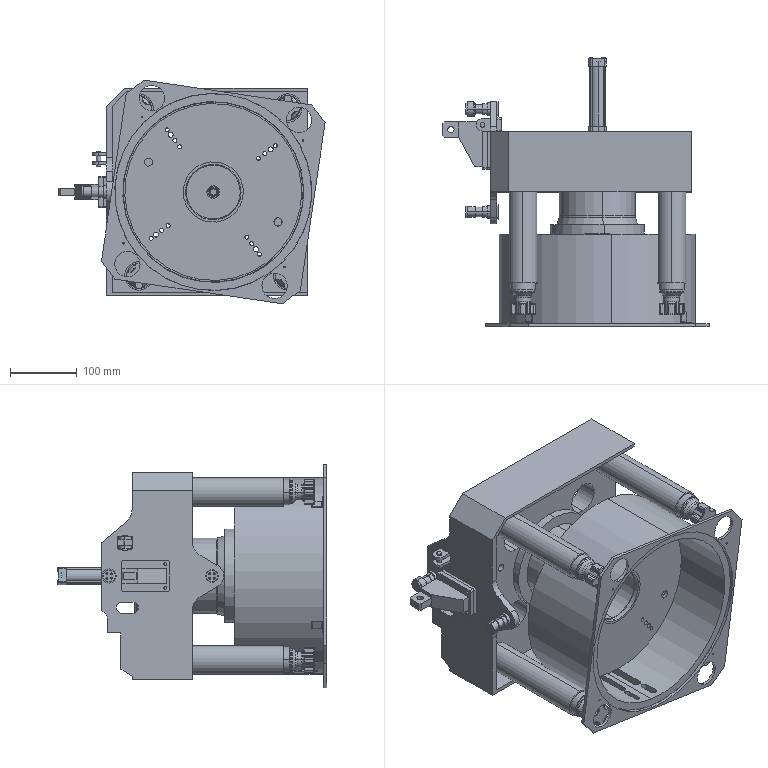Part | SolidWorks | 66 solids | 1913 faces | box 397.81 x 402.788 x 334.249 mm | volume 8465186 mm3 | cylinder 984 | plane 438 | torus 264 | cone 163 | spline 64 | commonest cylinder face diameters 2.484 x96 14.196 x79 0.946 x64 3.786 x64 5.915 x48 6.01 x40